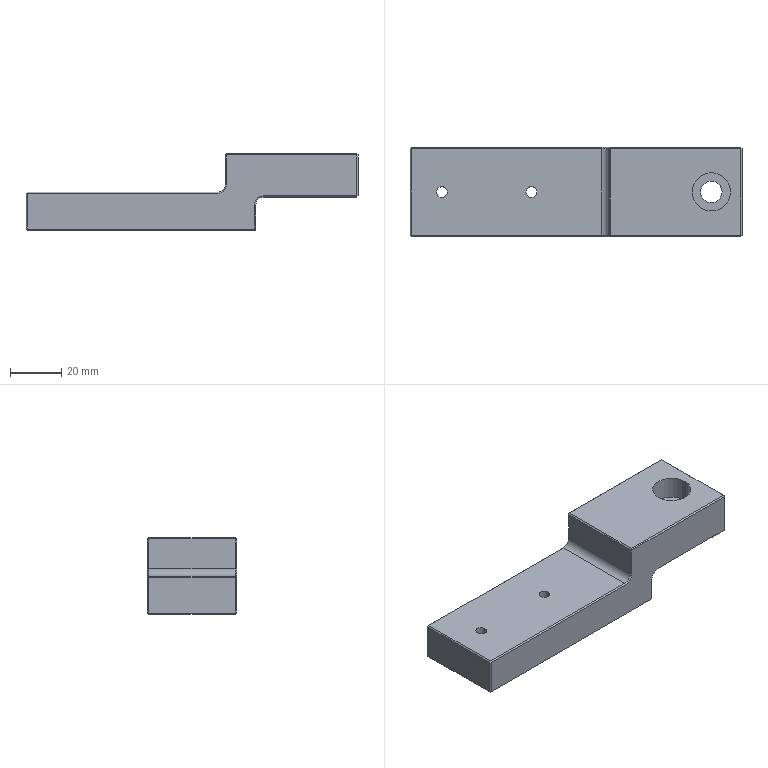Part | STEP file | 1 solid | 75 faces | box 130 x 35 x 30 mm | volume 74604 mm3 | plane 43 | cylinder 20 | cone 12 | commonest cylinder face diameters 2 x8 4.2 x4 6 x2 8.4 x2 15 x2 16 x2